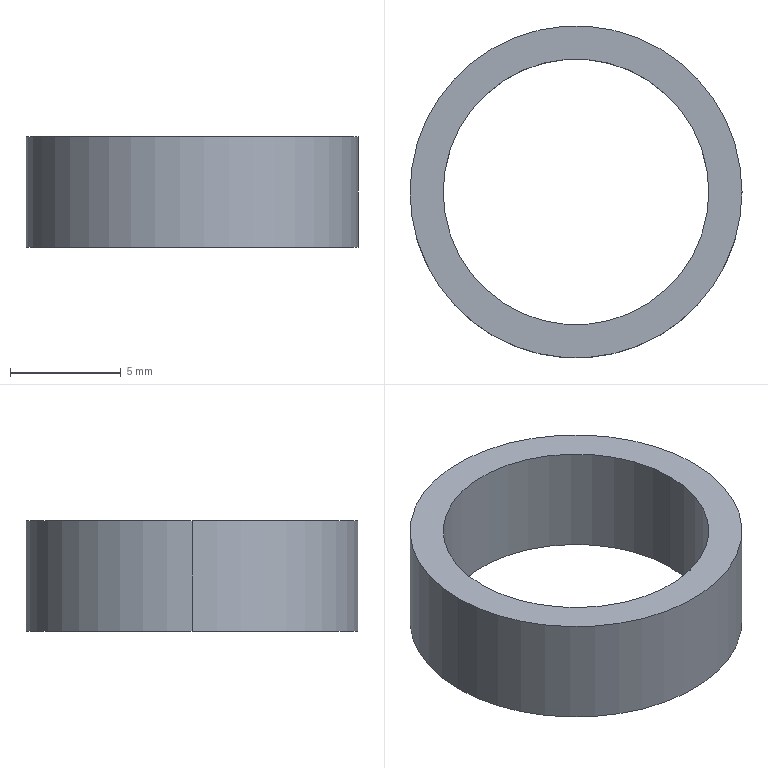Part | STEP file | 0230_Z_005_MRWZ12_3 | 1 solid | 6 faces | box 15 x 15 x 5 mm | volume 318.086 mm3 | cylinder 4 | plane 2 | commonest cylinder face diameters 12 x2 15 x2
STEP:
#1=CARTESIAN_POINT('',(0.,0.,0.));
#2=DIRECTION('',(0.,0.,1.));
#3=DIRECTION('',(1.,0.,0.));
#4=AXIS2_PLACEMENT_3D('',#1,#2,#3);
#5=CARTESIAN_POINT('',(-7.5,0.,5.5));
#6=VERTEX_POINT('',#5);
#7=CARTESIAN_POINT('',(7.5,0.,5.5));
#8=VERTEX_POINT('',#7);
#9=CARTESIAN_POINT('',(0.,0.,5.5));
#10=DIRECTION('',(0.,0.,-1.));
#11=DIRECTION('',(-1.,0.,0.));
#12=AXIS2_PLACEMENT_3D('',#9,#10,#11);
#13=CIRCLE('',#12,7.5);
#14=CARTESIAN_POINT('',(0.,0.,3.));
#15=DIRECTION('',(0.,0.,-1.));
#16=DIRECTION('',(-1.,0.,0.));
#17=AXIS2_PLACEMENT_3D('',#14,#15,#16);
#18=CYLINDRICAL_SURFACE('',#17,7.5);
#19=CARTESIAN_POINT('',(0.,-2.5));
#20=DIRECTION('',(1.,0.));
#21=VECTOR('',#20,1.);
#22=LINE('',#19,#21);
#23=(GEOMETRIC_REPRESENTATION_CONTEXT(2)PARAMETRIC_REPRESENTATION_CONTEXT()REPRESENTATION_CONTEXT('',''));
#24=DEFINITIONAL_REPRESENTATION('',(#22),#23);
#25=PCURVE('',#18,#24);
#26=CARTESIAN_POINT('',(0.,6.75,5.5));
#27=DIRECTION('',(0.,0.,1.));
#28=DIRECTION('',(1.,0.,0.));
#29=AXIS2_PLACEMENT_3D('',#26,#27,#28);
#30=PLANE('',#29);
#31=CARTESIAN_POINT('',(-7.5,-6.75));
#32=CARTESIAN_POINT('',(-7.5,6.24));
#33=CARTESIAN_POINT('',(3.75,-0.2548));
#34=CARTESIAN_POINT('',(15.,-6.75));
#35=CARTESIAN_POINT('',(3.75,-13.245));
#36=CARTESIAN_POINT('',(-7.5,-19.74));
#37=CARTESIAN_POINT('',(-7.5,-6.75));
#38=(BOUNDED_CURVE()B_SPLINE_CURVE(2,(#31,#32,#33,#34,#35,#36,#37),.UNSPECIFIED.,.T.,.F.)B_SPLINE_CURVE_WITH_KNOTS((1,2,2,2,2,1),(-2.094,0.,2.094,4.189,6.283,8.378),.UNSPECIFIED.)CURVE()GEOMETRIC_REPRESENTATION_ITEM()RATIONAL_B_SPLINE_CURVE((1.,0.5,1.,0.5,1.,0.5,1.))REPRESENTATION_ITEM(''));
#39=(GEOMETRIC_REPRESENTATION_CONTEXT(2)PARAMETRIC_REPRESENTATION_CONTEXT()REPRESENTATION_CONTEXT('',''));
#40=DEFINITIONAL_REPRESENTATION('',(#38),#39);
#41=PCURVE('',#30,#40);
#42=SURFACE_CURVE('',#13,(#25,#41),.PCURVE_S1.);
#43=EDGE_CURVE('',#6,#8,#42,.T.);
#44=ORIENTED_EDGE('',*,*,#43,.T.);
#45=CARTESIAN_POINT('',(7.5,0.,0.5));
#46=VERTEX_POINT('',#45);
#47=CARTESIAN_POINT('',(7.5,0.,3.));
#48=DIRECTION('',(0.,0.,-1.));
#49=VECTOR('',#48,1.);
#50=LINE('',#47,#49);
#51=CARTESIAN_POINT('',(3.142,0.));
#52=DIRECTION('',(0.,1.));
#53=VECTOR('',#52,1.);
#54=LINE('',#51,#53);
#55=(GEOMETRIC_REPRESENTATION_CONTEXT(2)PARAMETRIC_REPRESENTATION_CONTEXT()REPRESENTATION_CONTEXT('',''));
#56=DEFINITIONAL_REPRESENTATION('',(#54),#55);
#57=PCURVE('',#18,#56);
#58=CARTESIAN_POINT('',(0.,0.,3.));
#59=DIRECTION('',(0.,0.,-1.));
#60=DIRECTION('',(-1.,0.,0.));
#61=AXIS2_PLACEMENT_3D('',#58,#59,#60);
#62=CYLINDRICAL_SURFACE('',#61,7.5);
#63=CARTESIAN_POINT('',(3.142,0.));
#64=DIRECTION('',(0.,1.));
#65=VECTOR('',#64,1.);
#66=LINE('',#63,#65);
#67=(GEOMETRIC_REPRESENTATION_CONTEXT(2)PARAMETRIC_REPRESENTATION_CONTEXT()REPRESENTATION_CONTEXT('',''));
#68=DEFINITIONAL_REPRESENTATION('',(#66),#67);
#69=PCURVE('',#62,#68);
#70=SURFACE_CURVE('',#50,(#57,#69),.PCURVE_S1.);
#71=EDGE_CURVE('',#8,#46,#70,.T.);
#72=ORIENTED_EDGE('',*,*,#71,.T.);
#73=CARTESIAN_POINT('',(-7.5,0.,0.5));
#74=VERTEX_POINT('',#73);
#75=CARTESIAN_POINT('',(0.,0.,0.5));
#76=DIRECTION('',(0.,0.,1.));
#77=DIRECTION('',(-1.,0.,0.));
#78=AXIS2_PLACEMENT_3D('',#75,#76,#77);
#79=CIRCLE('',#78,7.5);
#80=CARTESIAN_POINT('',(6.283,2.5));
#81=DIRECTION('',(-1.,0.));
#82=VECTOR('',#81,1.);
#83=LINE('',#80,#82);
#84=(GEOMETRIC_REPRESENTATION_CONTEXT(2)PARAMETRIC_REPRESENTATION_CONTEXT()REPRESENTATION_CONTEXT('',''));
#85=DEFINITIONAL_REPRESENTATION('',(#83),#84);
#86=PCURVE('',#18,#85);
#87=CARTESIAN_POINT('',(0.,6.75,0.5));
#88=DIRECTION('',(0.,0.,-1.));
#89=DIRECTION('',(-1.,0.,0.));
#90=AXIS2_PLACEMENT_3D('',#87,#88,#89);
#91=PLANE('',#90);
#92=CARTESIAN_POINT('',(7.5,-6.75));
#93=CARTESIAN_POINT('',(7.5,-19.74));
#94=CARTESIAN_POINT('',(-3.75,-13.245));
#95=CARTESIAN_POINT('',(-15.,-6.75));
#96=CARTESIAN_POINT('',(-3.75,-0.2548));
#97=CARTESIAN_POINT('',(7.5,6.24));
#98=CARTESIAN_POINT('',(7.5,-6.75));
#99=(BOUNDED_CURVE()B_SPLINE_CURVE(2,(#92,#93,#94,#95,#96,#97,#98),.UNSPECIFIED.,.T.,.F.)B_SPLINE_CURVE_WITH_KNOTS((1,2,2,2,2,1),(-2.094,0.,2.094,4.189,6.283,8.378),.UNSPECIFIED.)CURVE()GEOMETRIC_REPRESENTATION_ITEM()RATIONAL_B_SPLINE_CURVE((1.,0.5,1.,0.5,1.,0.5,1.))REPRESENTATION_ITEM(''));
#100=(GEOMETRIC_REPRESENTATION_CONTEXT(2)PARAMETRIC_REPRESENTATION_CONTEXT()REPRESENTATION_CONTEXT('',''));
#101=DEFINITIONAL_REPRESENTATION('',(#99),#100);
#102=PCURVE('',#91,#101);
#103=SURFACE_CURVE('',#79,(#86,#102),.PCURVE_S1.);
#104=EDGE_CURVE('',#46,#74,#103,.T.);
#105=ORIENTED_EDGE('',*,*,#104,.T.);
#106=CARTESIAN_POINT('',(-7.5,0.,3.));
#107=DIRECTION('',(0.,0.,-1.));
#108=VECTOR('',#107,1.);
#109=LINE('',#106,#108);
#110=CARTESIAN_POINT('',(0.,0.));
#111=DIRECTION('',(0.,1.));
#112=VECTOR('',#111,1.);
#113=LINE('',#110,#112);
#114=(GEOMETRIC_REPRESENTATION_CONTEXT(2)PARAMETRIC_REPRESENTATION_CONTEXT()REPRESENTATION_CONTEXT('',''));
#115=DEFINITIONAL_REPRESENTATION('',(#113),#114);
#116=PCURVE('',#18,#115);
#117=CARTESIAN_POINT('',(6.283,0.));
#118=DIRECTION('',(0.,1.));
#119=VECTOR('',#118,1.);
#120=LINE('',#117,#119);
#121=(GEOMETRIC_REPRESENTATION_CONTEXT(2)PARAMETRIC_REPRESENTATION_CONTEXT()REPRESENTATION_CONTEXT('',''));
#122=DEFINITIONAL_REPRESENTATION('',(#120),#121);
#123=PCURVE('',#62,#122);
#124=SURFACE_CURVE('',#109,(#116,#123),.PCURVE_S1.);
#125=EDGE_CURVE('',#6,#74,#124,.T.);
#126=ORIENTED_EDGE('',*,*,#125,.F.);
#127=EDGE_LOOP('',(#44,#72,#105,#126));
#128=FACE_BOUND('',#127,.T.);
#129=ADVANCED_FACE('',(#128),#18,.T.);
#130=CARTESIAN_POINT('',(-6.,0.,5.5));
#131=VERTEX_POINT('',#130);
#132=CARTESIAN_POINT('',(-6.,0.,0.5));
#133=VERTEX_POINT('',#132);
#134=CARTESIAN_POINT('',(-6.,0.,3.));
#135=DIRECTION('',(0.,0.,-1.));
#136=VECTOR('',#135,1.);
#137=LINE('',#134,#136);
#138=CARTESIAN_POINT('',(0.,0.,3.));
#139=DIRECTION('',(0.,0.,-1.));
#140=DIRECTION('',(-1.,0.,0.));
#141=AXIS2_PLACEMENT_3D('',#138,#139,#140);
#142=CYLINDRICAL_SURFACE('',#141,6.);
#143=CARTESIAN_POINT('',(6.283,0.));
#144=DIRECTION('',(0.,1.));
#145=VECTOR('',#144,1.);
#146=LINE('',#143,#145);
#147=(GEOMETRIC_REPRESENTATION_CONTEXT(2)PARAMETRIC_REPRESENTATION_CONTEXT()REPRESENTATION_CONTEXT('',''));
#148=DEFINITIONAL_REPRESENTATION('',(#146),#147);
#149=PCURVE('',#142,#148);
#150=CARTESIAN_POINT('',(0.,0.,3.));
#151=DIRECTION('',(0.,0.,-1.));
#152=DIRECTION('',(-1.,0.,0.));
#153=AXIS2_PLACEMENT_3D('',#150,#151,#152);
#154=CYLINDRICAL_SURFACE('',#153,6.);
#155=CARTESIAN_POINT('',(0.,0.));
#156=DIRECTION('',(0.,1.));
#157=VECTOR('',#156,1.);
#158=LINE('',#155,#157);
#159=(GEOMETRIC_REPRESENTATION_CONTEXT(2)PARAMETRIC_REPRESENTATION_CONTEXT()REPRESENTATION_CONTEXT('',''));
#160=DEFINITIONAL_REPRESENTATION('',(#158),#159);
#161=PCURVE('',#154,#160);
#162=SURFACE_CURVE('',#137,(#149,#161),.PCURVE_S1.);
#163=EDGE_CURVE('',#131,#133,#162,.T.);
#164=ORIENTED_EDGE('',*,*,#163,.T.);
#165=CARTESIAN_POINT('',(6.,0.,0.5));
#166=VERTEX_POINT('',#165);
#167=CARTESIAN_POINT('',(0.,0.,0.5));
#168=DIRECTION('',(0.,0.,1.));
#169=DIRECTION('',(-1.,0.,0.));
#170=AXIS2_PLACEMENT_3D('',#167,#168,#169);
#171=CIRCLE('',#170,6.);
#172=CARTESIAN_POINT('',(6.283,2.5));
#173=DIRECTION('',(-1.,0.));
#174=VECTOR('',#173,1.);
#175=LINE('',#172,#174);
#176=(GEOMETRIC_REPRESENTATION_CONTEXT(2)PARAMETRIC_REPRESENTATION_CONTEXT()REPRESENTATION_CONTEXT('',''));
#177=DEFINITIONAL_REPRESENTATION('',(#175),#176);
#178=PCURVE('',#142,#177);
#179=CARTESIAN_POINT('',(6.,-6.75));
#180=CARTESIAN_POINT('',(6.,-17.142));
#181=CARTESIAN_POINT('',(-3.,-11.946));
#182=CARTESIAN_POINT('',(-12.,-6.75));
#183=CARTESIAN_POINT('',(-3.,-1.554));
#184=CARTESIAN_POINT('',(6.,3.642));
#185=CARTESIAN_POINT('',(6.,-6.75));
#186=(BOUNDED_CURVE()B_SPLINE_CURVE(2,(#179,#180,#181,#182,#183,#184,#185),.UNSPECIFIED.,.T.,.F.)B_SPLINE_CURVE_WITH_KNOTS((1,2,2,2,2,1),(-2.094,0.,2.094,4.189,6.283,8.378),.UNSPECIFIED.)CURVE()GEOMETRIC_REPRESENTATION_ITEM()RATIONAL_B_SPLINE_CURVE((1.,0.5,1.,0.5,1.,0.5,1.))REPRESENTATION_ITEM(''));
#187=(GEOMETRIC_REPRESENTATION_CONTEXT(2)PARAMETRIC_REPRESENTATION_CONTEXT()REPRESENTATION_CONTEXT('',''));
#188=DEFINITIONAL_REPRESENTATION('',(#186),#187);
#189=PCURVE('',#91,#188);
#190=SURFACE_CURVE('',#171,(#178,#189),.PCURVE_S1.);
#191=EDGE_CURVE('',#133,#166,#190,.T.);
#192=ORIENTED_EDGE('',*,*,#191,.T.);
#193=CARTESIAN_POINT('',(6.,0.,5.5));
#194=VERTEX_POINT('',#193);
#195=CARTESIAN_POINT('',(6.,0.,3.));
#196=DIRECTION('',(0.,0.,-1.));
#197=VECTOR('',#196,1.);
#198=LINE('',#195,#197);
#199=CARTESIAN_POINT('',(3.142,0.));
#200=DIRECTION('',(0.,1.));
#201=VECTOR('',#200,1.);
#202=LINE('',#199,#201);
#203=(GEOMETRIC_REPRESENTATION_CONTEXT(2)PARAMETRIC_REPRESENTATION_CONTEXT()REPRESENTATION_CONTEXT('',''));
#204=DEFINITIONAL_REPRESENTATION('',(#202),#203);
#205=PCURVE('',#142,#204);
#206=CARTESIAN_POINT('',(3.142,0.));
#207=DIRECTION('',(0.,1.));
#208=VECTOR('',#207,1.);
#209=LINE('',#206,#208);
#210=(GEOMETRIC_REPRESENTATION_CONTEXT(2)PARAMETRIC_REPRESENTATION_CONTEXT()REPRESENTATION_CONTEXT('',''));
#211=DEFINITIONAL_REPRESENTATION('',(#209),#210);
#212=PCURVE('',#154,#211);
#213=SURFACE_CURVE('',#198,(#205,#212),.PCURVE_S1.);
#214=EDGE_CURVE('',#194,#166,#213,.T.);
#215=ORIENTED_EDGE('',*,*,#214,.F.);
#216=CARTESIAN_POINT('',(0.,0.,5.5));
#217=DIRECTION('',(0.,0.,-1.));
#218=DIRECTION('',(-1.,0.,0.));
#219=AXIS2_PLACEMENT_3D('',#216,#217,#218);
#220=CIRCLE('',#219,6.);
#221=CARTESIAN_POINT('',(0.,-2.5));
#222=DIRECTION('',(1.,0.));
#223=VECTOR('',#222,1.);
#224=LINE('',#221,#223);
#225=(GEOMETRIC_REPRESENTATION_CONTEXT(2)PARAMETRIC_REPRESENTATION_CONTEXT()REPRESENTATION_CONTEXT('',''));
#226=DEFINITIONAL_REPRESENTATION('',(#224),#225);
#227=PCURVE('',#142,#226);
#228=CARTESIAN_POINT('',(-6.,-6.75));
#229=CARTESIAN_POINT('',(-6.,3.642));
#230=CARTESIAN_POINT('',(3.,-1.554));
#231=CARTESIAN_POINT('',(12.,-6.75));
#232=CARTESIAN_POINT('',(3.,-11.946));
#233=CARTESIAN_POINT('',(-6.,-17.142));
#234=CARTESIAN_POINT('',(-6.,-6.75));
#235=(BOUNDED_CURVE()B_SPLINE_CURVE(2,(#228,#229,#230,#231,#232,#233,#234),.UNSPECIFIED.,.T.,.F.)B_SPLINE_CURVE_WITH_KNOTS((1,2,2,2,2,1),(-2.094,0.,2.094,4.189,6.283,8.378),.UNSPECIFIED.)CURVE()GEOMETRIC_REPRESENTATION_ITEM()RATIONAL_B_SPLINE_CURVE((1.,0.5,1.,0.5,1.,0.5,1.))REPRESENTATION_ITEM(''));
#236=(GEOMETRIC_REPRESENTATION_CONTEXT(2)PARAMETRIC_REPRESENTATION_CONTEXT()REPRESENTATION_CONTEXT('',''));
#237=DEFINITIONAL_REPRESENTATION('',(#235),#236);
#238=PCURVE('',#30,#237);
#239=SURFACE_CURVE('',#220,(#227,#238),.PCURVE_S1.);
#240=EDGE_CURVE('',#194,#131,#239,.T.);
#241=ORIENTED_EDGE('',*,*,#240,.T.);
#242=EDGE_LOOP('',(#164,#192,#215,#241));
#243=FACE_BOUND('',#242,.F.);
#244=ADVANCED_FACE('',(#243),#142,.F.);
#245=ORIENTED_EDGE('',*,*,#71,.F.);
#246=CARTESIAN_POINT('',(0.,0.,5.5));
#247=DIRECTION('',(0.,0.,-1.));
#248=DIRECTION('',(-1.,0.,0.));
#249=AXIS2_PLACEMENT_3D('',#246,#247,#248);
#250=CIRCLE('',#249,7.5);
#251=CARTESIAN_POINT('',(0.,-2.5));
#252=DIRECTION('',(1.,0.));
#253=VECTOR('',#252,1.);
#254=LINE('',#251,#253);
#255=(GEOMETRIC_REPRESENTATION_CONTEXT(2)PARAMETRIC_REPRESENTATION_CONTEXT()REPRESENTATION_CONTEXT('',''));
#256=DEFINITIONAL_REPRESENTATION('',(#254),#255);
#257=PCURVE('',#62,#256);
#258=CARTESIAN_POINT('',(-7.5,-6.75));
#259=CARTESIAN_POINT('',(-7.5,6.24));
#260=CARTESIAN_POINT('',(3.75,-0.2548));
#261=CARTESIAN_POINT('',(15.,-6.75));
#262=CARTESIAN_POINT('',(3.75,-13.245));
#263=CARTESIAN_POINT('',(-7.5,-19.74));
#264=CARTESIAN_POINT('',(-7.5,-6.75));
#265=(BOUNDED_CURVE()B_SPLINE_CURVE(2,(#258,#259,#260,#261,#262,#263,#264),.UNSPECIFIED.,.T.,.F.)B_SPLINE_CURVE_WITH_KNOTS((1,2,2,2,2,1),(-2.094,0.,2.094,4.189,6.283,8.378),.UNSPECIFIED.)CURVE()GEOMETRIC_REPRESENTATION_ITEM()RATIONAL_B_SPLINE_CURVE((1.,0.5,1.,0.5,1.,0.5,1.))REPRESENTATION_ITEM(''));
#266=(GEOMETRIC_REPRESENTATION_CONTEXT(2)PARAMETRIC_REPRESENTATION_CONTEXT()REPRESENTATION_CONTEXT('',''));
#267=DEFINITIONAL_REPRESENTATION('',(#265),#266);
#268=PCURVE('',#30,#267);
#269=SURFACE_CURVE('',#250,(#257,#268),.PCURVE_S1.);
#270=EDGE_CURVE('',#8,#6,#269,.T.);
#271=ORIENTED_EDGE('',*,*,#270,.T.);
#272=ORIENTED_EDGE('',*,*,#125,.T.);
#273=CARTESIAN_POINT('',(0.,0.,0.5));
#274=DIRECTION('',(0.,0.,1.));
#275=DIRECTION('',(-1.,0.,0.));
#276=AXIS2_PLACEMENT_3D('',#273,#274,#275);
#277=CIRCLE('',#276,7.5);
#278=CARTESIAN_POINT('',(6.283,2.5));
#279=DIRECTION('',(-1.,0.));
#280=VECTOR('',#279,1.);
#281=LINE('',#278,#280);
#282=(GEOMETRIC_REPRESENTATION_CONTEXT(2)PARAMETRIC_REPRESENTATION_CONTEXT()REPRESENTATION_CONTEXT('',''));
#283=DEFINITIONAL_REPRESENTATION('',(#281),#282);
#284=PCURVE('',#62,#283);
#285=CARTESIAN_POINT('',(7.5,-6.75));
#286=CARTESIAN_POINT('',(7.5,-19.74));
#287=CARTESIAN_POINT('',(-3.75,-13.245));
#288=CARTESIAN_POINT('',(-15.,-6.75));
#289=CARTESIAN_POINT('',(-3.75,-0.2548));
#290=CARTESIAN_POINT('',(7.5,6.24));
#291=CARTESIAN_POINT('',(7.5,-6.75));
#292=(BOUNDED_CURVE()B_SPLINE_CURVE(2,(#285,#286,#287,#288,#289,#290,#291),.UNSPECIFIED.,.T.,.F.)B_SPLINE_CURVE_WITH_KNOTS((1,2,2,2,2,1),(-2.094,0.,2.094,4.189,6.283,8.378),.UNSPECIFIED.)CURVE()GEOMETRIC_REPRESENTATION_ITEM()RATIONAL_B_SPLINE_CURVE((1.,0.5,1.,0.5,1.,0.5,1.))REPRESENTATION_ITEM(''));
#293=(GEOMETRIC_REPRESENTATION_CONTEXT(2)PARAMETRIC_REPRESENTATION_CONTEXT()REPRESENTATION_CONTEXT('',''));
#294=DEFINITIONAL_REPRESENTATION('',(#292),#293);
#295=PCURVE('',#91,#294);
#296=SURFACE_CURVE('',#277,(#284,#295),.PCURVE_S1.);
#297=EDGE_CURVE('',#74,#46,#296,.T.);
#298=ORIENTED_EDGE('',*,*,#297,.T.);
#299=EDGE_LOOP('',(#245,#271,#272,#298));
#300=FACE_BOUND('',#299,.T.);
#301=ADVANCED_FACE('',(#300),#62,.T.);
#302=ORIENTED_EDGE('',*,*,#43,.F.);
#303=ORIENTED_EDGE('',*,*,#270,.F.);
#304=EDGE_LOOP('',(#302,#303));
#305=FACE_BOUND('',#304,.T.);
#306=CARTESIAN_POINT('',(0.,0.,5.5));
#307=DIRECTION('',(0.,0.,-1.));
#308=DIRECTION('',(-1.,0.,0.));
#309=AXIS2_PLACEMENT_3D('',#306,#307,#308);
#310=CIRCLE('',#309,6.);
#311=CARTESIAN_POINT('',(-6.,-6.75));
#312=CARTESIAN_POINT('',(-6.,3.642));
#313=CARTESIAN_POINT('',(3.,-1.554));
#314=CARTESIAN_POINT('',(12.,-6.75));
#315=CARTESIAN_POINT('',(3.,-11.946));
#316=CARTESIAN_POINT('',(-6.,-17.142));
#317=CARTESIAN_POINT('',(-6.,-6.75));
#318=(BOUNDED_CURVE()B_SPLINE_CURVE(2,(#311,#312,#313,#314,#315,#316,#317),.UNSPECIFIED.,.T.,.F.)B_SPLINE_CURVE_WITH_KNOTS((1,2,2,2,2,1),(-2.094,0.,2.094,4.189,6.283,8.378),.UNSPECIFIED.)CURVE()GEOMETRIC_REPRESENTATION_ITEM()RATIONAL_B_SPLINE_CURVE((1.,0.5,1.,0.5,1.,0.5,1.))REPRESENTATION_ITEM(''));
#319=(GEOMETRIC_REPRESENTATION_CONTEXT(2)PARAMETRIC_REPRESENTATION_CONTEXT()REPRESENTATION_CONTEXT('',''));
#320=DEFINITIONAL_REPRESENTATION('',(#318),#319);
#321=PCURVE('',#30,#320);
#322=CARTESIAN_POINT('',(0.,-2.5));
#323=DIRECTION('',(1.,0.));
#324=VECTOR('',#323,1.);
#325=LINE('',#322,#324);
#326=(GEOMETRIC_REPRESENTATION_CONTEXT(2)PARAMETRIC_REPRESENTATION_CONTEXT()REPRESENTATION_CONTEXT('',''));
#327=DEFINITIONAL_REPRESENTATION('',(#325),#326);
#328=PCURVE('',#154,#327);
#329=SURFACE_CURVE('',#310,(#321,#328),.PCURVE_S1.);
#330=EDGE_CURVE('',#131,#194,#329,.T.);
#331=ORIENTED_EDGE('',*,*,#330,.T.);
#332=ORIENTED_EDGE('',*,*,#240,.T.);
#333=EDGE_LOOP('',(#331,#332));
#334=FACE_BOUND('',#333,.T.);
#335=ADVANCED_FACE('',(#305,#334),#30,.T.);
#336=ORIENTED_EDGE('',*,*,#191,.T.);
#337=CARTESIAN_POINT('',(0.,0.,0.5));
#338=DIRECTION('',(0.,0.,1.));
#339=DIRECTION('',(-1.,0.,0.));
#340=AXIS2_PLACEMENT_3D('',#337,#338,#339);
#341=CIRCLE('',#340,6.);
#342=CARTESIAN_POINT('',(6.,-6.75));
#343=CARTESIAN_POINT('',(6.,-17.142));
#344=CARTESIAN_POINT('',(-3.,-11.946));
#345=CARTESIAN_POINT('',(-12.,-6.75));
#346=CARTESIAN_POINT('',(-3.,-1.554));
#347=CARTESIAN_POINT('',(6.,3.642));
#348=CARTESIAN_POINT('',(6.,-6.75));
#349=(BOUNDED_CURVE()B_SPLINE_CURVE(2,(#342,#343,#344,#345,#346,#347,#348),.UNSPECIFIED.,.T.,.F.)B_SPLINE_CURVE_WITH_KNOTS((1,2,2,2,2,1),(-2.094,0.,2.094,4.189,6.283,8.378),.UNSPECIFIED.)CURVE()GEOMETRIC_REPRESENTATION_ITEM()RATIONAL_B_SPLINE_CURVE((1.,0.5,1.,0.5,1.,0.5,1.))REPRESENTATION_ITEM(''));
#350=(GEOMETRIC_REPRESENTATION_CONTEXT(2)PARAMETRIC_REPRESENTATION_CONTEXT()REPRESENTATION_CONTEXT('',''));
#351=DEFINITIONAL_REPRESENTATION('',(#349),#350);
#352=PCURVE('',#91,#351);
#353=CARTESIAN_POINT('',(6.283,2.5));
#354=DIRECTION('',(-1.,0.));
#355=VECTOR('',#354,1.);
#356=LINE('',#353,#355);
#357=(GEOMETRIC_REPRESENTATION_CONTEXT(2)PARAMETRIC_REPRESENTATION_CONTEXT()REPRESENTATION_CONTEXT('',''));
#358=DEFINITIONAL_REPRESENTATION('',(#356),#357);
#359=PCURVE('',#154,#358);
#360=SURFACE_CURVE('',#341,(#352,#359),.PCURVE_S1.);
#361=EDGE_CURVE('',#166,#133,#360,.T.);
#362=ORIENTED_EDGE('',*,*,#361,.T.);
#363=EDGE_LOOP('',(#336,#362));
#364=FACE_BOUND('',#363,.T.);
#365=ORIENTED_EDGE('',*,*,#297,.F.);
#366=ORIENTED_EDGE('',*,*,#104,.F.);
#367=EDGE_LOOP('',(#365,#366));
#368=FACE_BOUND('',#367,.T.);
#369=ADVANCED_FACE('',(#364,#368),#91,.T.);
#370=ORIENTED_EDGE('',*,*,#361,.T.);
#371=ORIENTED_EDGE('',*,*,#163,.F.);
#372=ORIENTED_EDGE('',*,*,#330,.T.);
#373=ORIENTED_EDGE('',*,*,#214,.T.);
#374=EDGE_LOOP('',(#370,#371,#372,#373));
#375=FACE_BOUND('',#374,.F.);
#376=ADVANCED_FACE('',(#375),#154,.F.);
#377=CLOSED_SHELL('',(#129,#244,#301,#335,#369,#376));
#378=MANIFOLD_SOLID_BREP('',#377);
#379=(LENGTH_UNIT()NAMED_UNIT(*)SI_UNIT(.MILLI.,.METRE.));
#380=UNCERTAINTY_MEASURE_WITH_UNIT(LENGTH_MEASURE(0.0000001),#379,'','');
#381=(NAMED_UNIT(*)PLANE_ANGLE_UNIT()SI_UNIT($,.RADIAN.));
#382=(NAMED_UNIT(*)SI_UNIT($,.STERADIAN.)SOLID_ANGLE_UNIT());
#383=(GEOMETRIC_REPRESENTATION_CONTEXT(3)GLOBAL_UNCERTAINTY_ASSIGNED_CONTEXT((#380))GLOBAL_UNIT_ASSIGNED_CONTEXT((#379,#381,#382))REPRESENTATION_CONTEXT('',''));
#384=ADVANCED_BREP_SHAPE_REPRESENTATION('',(#4,#378),#383);